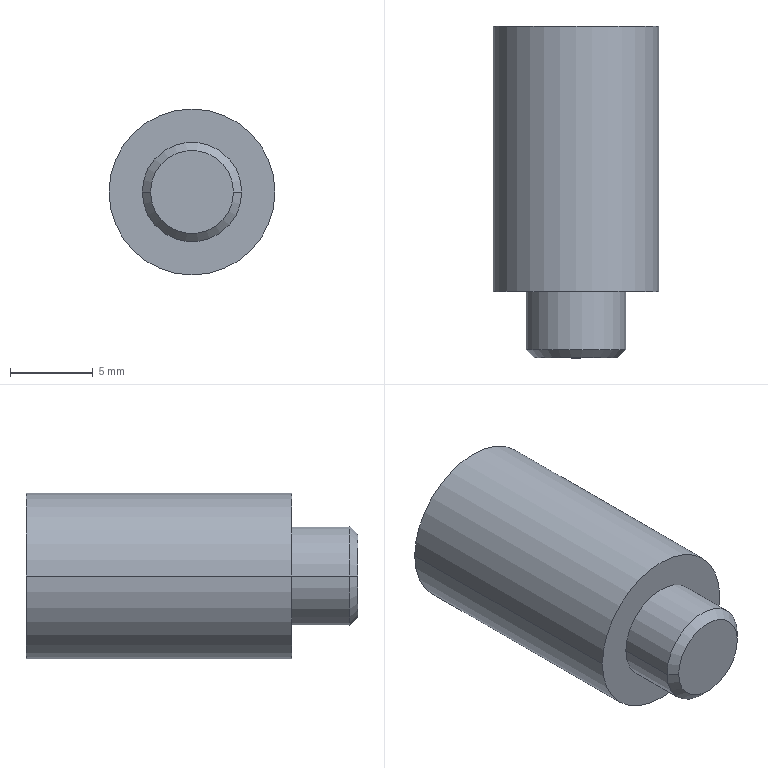Part | SolidWorks | features Chamfer 1, Revolution 1 | 1 solid | 9 faces | box 10 x 20 x 10 mm | volume 1368 mm3 | cylinder 4 | plane 3 | cone 2 | commonest cylinder face diameters 6 x2 10 x2
STEP:
#1=CARTESIAN_POINT('',(2.5,-20.,0.));
#2=VERTEX_POINT('',#1);
#3=CARTESIAN_POINT('',(-2.5,-20.,0.));
#4=VERTEX_POINT('',#3);
#5=CARTESIAN_POINT('',(0.,-20.,0.));
#6=DIRECTION('',(0.,-1.,0.));
#7=DIRECTION('',(1.,0.,0.));
#8=AXIS2_PLACEMENT_3D('',#5,#6,#7);
#9=CIRCLE('',#8,2.5);
#10=EDGE_CURVE('',#2,#4,#9,.T.);
#11=ORIENTED_EDGE('',*,*,#10,.F.);
#12=CARTESIAN_POINT('',(3.,-19.5,0.));
#13=VERTEX_POINT('',#12);
#14=CARTESIAN_POINT('',(2.5,-20.,0.));
#15=DIRECTION('',(0.7071,0.7071,0.));
#16=VECTOR('',#15,1000.);
#17=LINE('',#14,#16);
#18=EDGE_CURVE('',#2,#13,#17,.T.);
#19=ORIENTED_EDGE('',*,*,#18,.T.);
#20=CARTESIAN_POINT('',(-3.,-19.5,0.));
#21=VERTEX_POINT('',#20);
#22=CARTESIAN_POINT('',(0.,-19.5,0.));
#23=DIRECTION('',(0.,1.,0.));
#24=DIRECTION('',(1.,0.,0.));
#25=AXIS2_PLACEMENT_3D('',#22,#23,#24);
#26=CIRCLE('',#25,3.);
#27=EDGE_CURVE('',#21,#13,#26,.T.);
#28=ORIENTED_EDGE('',*,*,#27,.F.);
#29=CARTESIAN_POINT('',(-2.5,-20.,0.));
#30=DIRECTION('',(-0.7071,0.7071,0.));
#31=VECTOR('',#30,1000.);
#32=LINE('',#29,#31);
#33=EDGE_CURVE('',#4,#21,#32,.T.);
#34=ORIENTED_EDGE('',*,*,#33,.F.);
#35=EDGE_LOOP('',(#11,#19,#28,#34));
#36=FACE_OUTER_BOUND('',#35,.T.);
#37=CARTESIAN_POINT('',(0.,-20.,0.));
#38=DIRECTION('',(0.,1.,0.));
#39=DIRECTION('',(-1.,0.,0.));
#40=AXIS2_PLACEMENT_3D('',#37,#38,#39);
#41=CONICAL_SURFACE('',#40,2.5,0.7854);
#42=ADVANCED_FACE('',(#36),#41,.T.);
#43=CARTESIAN_POINT('',(3.,-16.,0.));
#44=VERTEX_POINT('',#43);
#45=CARTESIAN_POINT('',(-3.,-16.,0.));
#46=VERTEX_POINT('',#45);
#47=CARTESIAN_POINT('',(0.,-16.,0.));
#48=DIRECTION('',(0.,-1.,0.));
#49=DIRECTION('',(1.,0.,0.));
#50=AXIS2_PLACEMENT_3D('',#47,#48,#49);
#51=CIRCLE('',#50,3.);
#52=EDGE_CURVE('',#44,#46,#51,.T.);
#53=ORIENTED_EDGE('',*,*,#52,.T.);
#54=CARTESIAN_POINT('',(-3.,-324.965,0.));
#55=DIRECTION('',(0.,-1.,0.));
#56=VECTOR('',#55,1000.);
#57=LINE('',#54,#56);
#58=EDGE_CURVE('',#46,#21,#57,.T.);
#59=ORIENTED_EDGE('',*,*,#58,.T.);
#60=ORIENTED_EDGE('',*,*,#27,.T.);
#61=CARTESIAN_POINT('',(3.,-324.965,0.));
#62=DIRECTION('',(0.,-1.,0.));
#63=VECTOR('',#62,1000.);
#64=LINE('',#61,#63);
#65=EDGE_CURVE('',#44,#13,#64,.T.);
#66=ORIENTED_EDGE('',*,*,#65,.F.);
#67=EDGE_LOOP('',(#53,#59,#60,#66));
#68=FACE_OUTER_BOUND('',#67,.T.);
#69=CARTESIAN_POINT('',(0.,-324.965,0.));
#70=DIRECTION('',(0.,-1.,0.));
#71=DIRECTION('',(1.,0.,0.));
#72=AXIS2_PLACEMENT_3D('',#69,#70,#71);
#73=CYLINDRICAL_SURFACE('',#72,3.);
#74=ADVANCED_FACE('',(#68),#73,.T.);
#75=CARTESIAN_POINT('',(5.,0.,0.));
#76=VERTEX_POINT('',#75);
#77=CARTESIAN_POINT('',(-5.,0.,0.));
#78=VERTEX_POINT('',#77);
#79=CARTESIAN_POINT('',(0.,0.,0.));
#80=DIRECTION('',(0.,-1.,0.));
#81=DIRECTION('',(1.,0.,0.));
#82=AXIS2_PLACEMENT_3D('',#79,#80,#81);
#83=CIRCLE('',#82,5.);
#84=EDGE_CURVE('',#76,#78,#83,.T.);
#85=ORIENTED_EDGE('',*,*,#84,.T.);
#86=CARTESIAN_POINT('',(-5.,-16.,0.));
#87=VERTEX_POINT('',#86);
#88=CARTESIAN_POINT('',(-5.,-324.965,0.));
#89=DIRECTION('',(0.,-1.,0.));
#90=VECTOR('',#89,1000.);
#91=LINE('',#88,#90);
#92=EDGE_CURVE('',#78,#87,#91,.T.);
#93=ORIENTED_EDGE('',*,*,#92,.T.);
#94=CARTESIAN_POINT('',(5.,-16.,0.));
#95=VERTEX_POINT('',#94);
#96=CARTESIAN_POINT('',(0.,-16.,0.));
#97=DIRECTION('',(0.,-1.,0.));
#98=DIRECTION('',(1.,0.,0.));
#99=AXIS2_PLACEMENT_3D('',#96,#97,#98);
#100=CIRCLE('',#99,5.);
#101=EDGE_CURVE('',#95,#87,#100,.T.);
#102=ORIENTED_EDGE('',*,*,#101,.F.);
#103=CARTESIAN_POINT('',(5.,-324.965,0.));
#104=DIRECTION('',(0.,-1.,0.));
#105=VECTOR('',#104,1000.);
#106=LINE('',#103,#105);
#107=EDGE_CURVE('',#76,#95,#106,.T.);
#108=ORIENTED_EDGE('',*,*,#107,.F.);
#109=EDGE_LOOP('',(#85,#93,#102,#108));
#110=FACE_OUTER_BOUND('',#109,.T.);
#111=CARTESIAN_POINT('',(0.,-324.965,0.));
#112=DIRECTION('',(0.,-1.,0.));
#113=DIRECTION('',(1.,0.,0.));
#114=AXIS2_PLACEMENT_3D('',#111,#112,#113);
#115=CYLINDRICAL_SURFACE('',#114,5.);
#116=ADVANCED_FACE('',(#110),#115,.T.);
#117=ORIENTED_EDGE('',*,*,#84,.F.);
#118=CARTESIAN_POINT('',(0.,0.,0.));
#119=DIRECTION('',(0.,-1.,0.));
#120=DIRECTION('',(1.,0.,0.));
#121=AXIS2_PLACEMENT_3D('',#118,#119,#120);
#122=CIRCLE('',#121,5.);
#123=EDGE_CURVE('',#78,#76,#122,.T.);
#124=ORIENTED_EDGE('',*,*,#123,.F.);
#125=EDGE_LOOP('',(#117,#124));
#126=FACE_OUTER_BOUND('',#125,.T.);
#127=CARTESIAN_POINT('',(0.,0.,0.));
#128=DIRECTION('',(0.,1.,0.));
#129=DIRECTION('',(-1.,0.,0.));
#130=AXIS2_PLACEMENT_3D('',#127,#128,#129);
#131=PLANE('',#130);
#132=ADVANCED_FACE('',(#126),#131,.T.);
#133=ORIENTED_EDGE('',*,*,#92,.F.);
#134=ORIENTED_EDGE('',*,*,#123,.T.);
#135=ORIENTED_EDGE('',*,*,#107,.T.);
#136=CARTESIAN_POINT('',(0.,-16.,0.));
#137=DIRECTION('',(0.,-1.,0.));
#138=DIRECTION('',(1.,0.,0.));
#139=AXIS2_PLACEMENT_3D('',#136,#137,#138);
#140=CIRCLE('',#139,5.);
#141=EDGE_CURVE('',#87,#95,#140,.T.);
#142=ORIENTED_EDGE('',*,*,#141,.F.);
#143=EDGE_LOOP('',(#133,#134,#135,#142));
#144=FACE_OUTER_BOUND('',#143,.T.);
#145=CARTESIAN_POINT('',(0.,-324.965,0.));
#146=DIRECTION('',(0.,-1.,0.));
#147=DIRECTION('',(1.,0.,0.));
#148=AXIS2_PLACEMENT_3D('',#145,#146,#147);
#149=CYLINDRICAL_SURFACE('',#148,5.);
#150=ADVANCED_FACE('',(#144),#149,.T.);
#151=ORIENTED_EDGE('',*,*,#101,.T.);
#152=ORIENTED_EDGE('',*,*,#141,.T.);
#153=EDGE_LOOP('',(#151,#152));
#154=FACE_OUTER_BOUND('',#153,.T.);
#155=ORIENTED_EDGE('',*,*,#52,.F.);
#156=CARTESIAN_POINT('',(0.,-16.,0.));
#157=DIRECTION('',(0.,-1.,0.));
#158=DIRECTION('',(1.,0.,0.));
#159=AXIS2_PLACEMENT_3D('',#156,#157,#158);
#160=CIRCLE('',#159,3.);
#161=EDGE_CURVE('',#46,#44,#160,.T.);
#162=ORIENTED_EDGE('',*,*,#161,.F.);
#163=EDGE_LOOP('',(#155,#162));
#164=FACE_BOUND('',#163,.T.);
#165=CARTESIAN_POINT('',(5.,-16.,0.));
#166=DIRECTION('',(0.,-1.,0.));
#167=DIRECTION('',(1.,0.,0.));
#168=AXIS2_PLACEMENT_3D('',#165,#166,#167);
#169=PLANE('',#168);
#170=ADVANCED_FACE('',(#154,#164),#169,.T.);
#171=ORIENTED_EDGE('',*,*,#58,.F.);
#172=ORIENTED_EDGE('',*,*,#161,.T.);
#173=ORIENTED_EDGE('',*,*,#65,.T.);
#174=CARTESIAN_POINT('',(0.,-19.5,0.));
#175=DIRECTION('',(0.,1.,0.));
#176=DIRECTION('',(1.,0.,0.));
#177=AXIS2_PLACEMENT_3D('',#174,#175,#176);
#178=CIRCLE('',#177,3.);
#179=EDGE_CURVE('',#13,#21,#178,.T.);
#180=ORIENTED_EDGE('',*,*,#179,.T.);
#181=EDGE_LOOP('',(#171,#172,#173,#180));
#182=FACE_OUTER_BOUND('',#181,.T.);
#183=CARTESIAN_POINT('',(0.,-324.965,0.));
#184=DIRECTION('',(0.,-1.,0.));
#185=DIRECTION('',(1.,0.,0.));
#186=AXIS2_PLACEMENT_3D('',#183,#184,#185);
#187=CYLINDRICAL_SURFACE('',#186,3.);
#188=ADVANCED_FACE('',(#182),#187,.T.);
#189=CARTESIAN_POINT('',(0.,-20.,0.));
#190=DIRECTION('',(0.,-1.,0.));
#191=DIRECTION('',(1.,0.,0.));
#192=AXIS2_PLACEMENT_3D('',#189,#190,#191);
#193=CIRCLE('',#192,2.5);
#194=EDGE_CURVE('',#4,#2,#193,.T.);
#195=ORIENTED_EDGE('',*,*,#194,.T.);
#196=ORIENTED_EDGE('',*,*,#10,.T.);
#197=EDGE_LOOP('',(#195,#196));
#198=FACE_OUTER_BOUND('',#197,.T.);
#199=CARTESIAN_POINT('',(3.,-20.,0.));
#200=DIRECTION('',(0.,-1.,0.));
#201=DIRECTION('',(1.,0.,0.));
#202=AXIS2_PLACEMENT_3D('',#199,#200,#201);
#203=PLANE('',#202);
#204=ADVANCED_FACE('',(#198),#203,.T.);
#205=ORIENTED_EDGE('',*,*,#18,.F.);
#206=ORIENTED_EDGE('',*,*,#194,.F.);
#207=ORIENTED_EDGE('',*,*,#33,.T.);
#208=ORIENTED_EDGE('',*,*,#179,.F.);
#209=EDGE_LOOP('',(#205,#206,#207,#208));
#210=FACE_OUTER_BOUND('',#209,.T.);
#211=CARTESIAN_POINT('',(0.,-20.,0.));
#212=DIRECTION('',(0.,1.,0.));
#213=DIRECTION('',(-1.,0.,0.));
#214=AXIS2_PLACEMENT_3D('',#211,#212,#213);
#215=CONICAL_SURFACE('',#214,2.5,0.7854);
#216=ADVANCED_FACE('',(#210),#215,.T.);
#217=CLOSED_SHELL('',(#42,#74,#116,#132,#150,#170,#188,#204,#216));
#218=MANIFOLD_SOLID_BREP('',#217);
#219=CARTESIAN_POINT('',(0.,0.,0.));
#220=DIRECTION('',(0.,0.,1.));
#221=DIRECTION('',(1.,0.,0.));
#222=AXIS2_PLACEMENT_3D('',#219,#220,#221);
#223=(LENGTH_UNIT()NAMED_UNIT(*)SI_UNIT(.MILLI.,.METRE.));
#224=UNCERTAINTY_MEASURE_WITH_UNIT(LENGTH_MEASURE(0.00001),#223,'','');
#225=(NAMED_UNIT(*)PLANE_ANGLE_UNIT()SI_UNIT($,.RADIAN.));
#226=(NAMED_UNIT(*)SI_UNIT($,.STERADIAN.)SOLID_ANGLE_UNIT());
#227=(GEOMETRIC_REPRESENTATION_CONTEXT(3)GLOBAL_UNCERTAINTY_ASSIGNED_CONTEXT((#224))GLOBAL_UNIT_ASSIGNED_CONTEXT((#223,#225,#226))REPRESENTATION_CONTEXT('',''));
#228=ADVANCED_BREP_SHAPE_REPRESENTATION('',(#218,#222),#227);